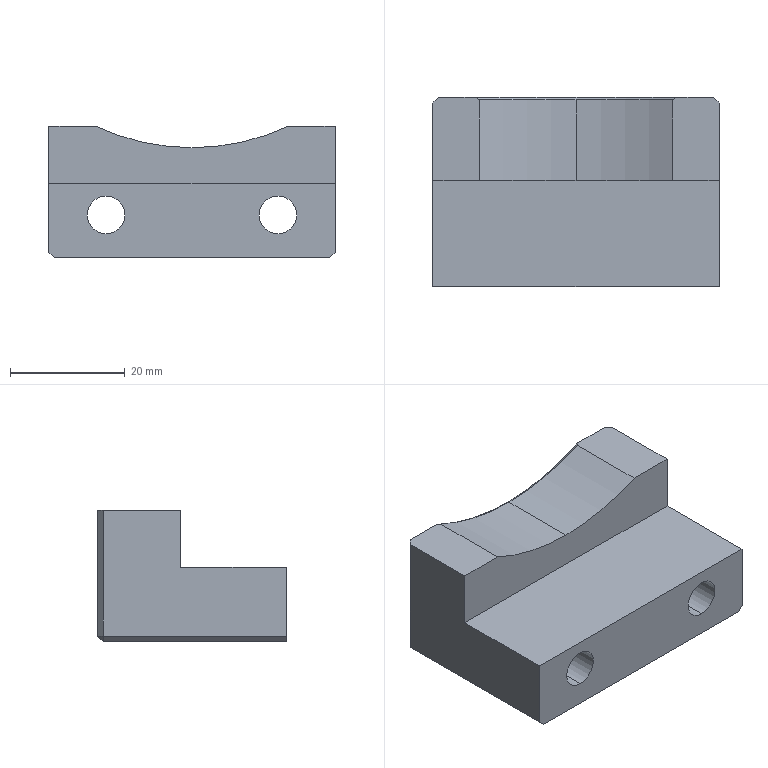Part | STEP file | PN_0004 Default | 1 solid | 29 faces | box 50 x 33 x 23 mm | volume 24275 mm3 | plane 18 | cylinder 10 | cone 1 | commonest cylinder face diameters 6.6 x4 11 x4 79.5 x2
STEP:
#1=CARTESIAN_POINT('',(16.854,32.57,3.));
#2=VERTEX_POINT('',#1);
#3=CARTESIAN_POINT('',(0.,32.57,-0.75));
#4=VERTEX_POINT('',#3);
#5=CARTESIAN_POINT('',(0.,32.57,39.));
#6=DIRECTION('',(0.,1.,0.));
#7=DIRECTION('',(0.,0.,-1.));
#8=AXIS2_PLACEMENT_3D('',#5,#6,#7);
#9=CIRCLE('',#8,39.75);
#10=EDGE_CURVE('',#2,#4,#9,.T.);
#11=ORIENTED_EDGE('',*,*,#10,.T.);
#12=CARTESIAN_POINT('',(0.,18.5,-0.75));
#13=VERTEX_POINT('',#12);
#14=CARTESIAN_POINT('',(0.,77.5,-0.75));
#15=DIRECTION('',(0.,-1.,0.));
#16=VECTOR('',#15,1000.);
#17=LINE('',#14,#16);
#18=EDGE_CURVE('',#4,#13,#17,.T.);
#19=ORIENTED_EDGE('',*,*,#18,.T.);
#20=CARTESIAN_POINT('',(16.854,18.5,3.));
#21=VERTEX_POINT('',#20);
#22=CARTESIAN_POINT('',(0.,18.5,39.));
#23=DIRECTION('',(0.,-1.,0.));
#24=DIRECTION('',(0.,0.,-1.));
#25=AXIS2_PLACEMENT_3D('',#22,#23,#24);
#26=CIRCLE('',#25,39.75);
#27=EDGE_CURVE('',#13,#21,#26,.T.);
#28=ORIENTED_EDGE('',*,*,#27,.T.);
#29=CARTESIAN_POINT('',(16.854,77.5,3.));
#30=DIRECTION('',(0.,-1.,0.));
#31=VECTOR('',#30,1000.);
#32=LINE('',#29,#31);
#33=EDGE_CURVE('',#2,#21,#32,.T.);
#34=ORIENTED_EDGE('',*,*,#33,.F.);
#35=EDGE_LOOP('',(#11,#19,#28,#34));
#36=FACE_OUTER_BOUND('',#35,.T.);
#37=CARTESIAN_POINT('',(0.,77.5,39.));
#38=DIRECTION('',(0.,-1.,0.));
#39=DIRECTION('',(0.,0.,-1.));
#40=AXIS2_PLACEMENT_3D('',#37,#38,#39);
#41=CYLINDRICAL_SURFACE('',#40,39.75);
#42=ADVANCED_FACE('',(#36),#41,.F.);
#43=CARTESIAN_POINT('',(-15.,26.,-18.));
#44=VERTEX_POINT('',#43);
#45=CARTESIAN_POINT('',(-15.,26.,-7.));
#46=VERTEX_POINT('',#45);
#47=CARTESIAN_POINT('',(-15.,26.,-12.5));
#48=DIRECTION('',(0.,1.,0.));
#49=DIRECTION('',(0.,0.,1.));
#50=AXIS2_PLACEMENT_3D('',#47,#48,#49);
#51=CIRCLE('',#50,5.5);
#52=EDGE_CURVE('',#44,#46,#51,.T.);
#53=ORIENTED_EDGE('',*,*,#52,.F.);
#54=CARTESIAN_POINT('',(-15.,33.,-18.));
#55=VERTEX_POINT('',#54);
#56=CARTESIAN_POINT('',(-15.,33.,-18.));
#57=DIRECTION('',(0.,1.,0.));
#58=VECTOR('',#57,1000.);
#59=LINE('',#56,#58);
#60=EDGE_CURVE('',#44,#55,#59,.T.);
#61=ORIENTED_EDGE('',*,*,#60,.T.);
#62=CARTESIAN_POINT('',(-15.,33.,-7.));
#63=VERTEX_POINT('',#62);
#64=CARTESIAN_POINT('',(-15.,33.,-12.5));
#65=DIRECTION('',(0.,1.,0.));
#66=DIRECTION('',(0.,0.,1.));
#67=AXIS2_PLACEMENT_3D('',#64,#65,#66);
#68=CIRCLE('',#67,5.5);
#69=EDGE_CURVE('',#55,#63,#68,.T.);
#70=ORIENTED_EDGE('',*,*,#69,.T.);
#71=CARTESIAN_POINT('',(-15.,33.,-7.));
#72=DIRECTION('',(0.,1.,0.));
#73=VECTOR('',#72,1000.);
#74=LINE('',#71,#73);
#75=EDGE_CURVE('',#46,#63,#74,.T.);
#76=ORIENTED_EDGE('',*,*,#75,.F.);
#77=EDGE_LOOP('',(#53,#61,#70,#76));
#78=FACE_OUTER_BOUND('',#77,.T.);
#79=CARTESIAN_POINT('',(-15.,33.,-12.5));
#80=DIRECTION('',(0.,1.,0.));
#81=DIRECTION('',(0.,0.,1.));
#82=AXIS2_PLACEMENT_3D('',#79,#80,#81);
#83=CYLINDRICAL_SURFACE('',#82,5.5);
#84=ADVANCED_FACE('',(#78),#83,.F.);
#85=CARTESIAN_POINT('',(-15.,0.,-15.8));
#86=VERTEX_POINT('',#85);
#87=CARTESIAN_POINT('',(-15.,0.,-9.2));
#88=VERTEX_POINT('',#87);
#89=CARTESIAN_POINT('',(-15.,0.,-12.5));
#90=DIRECTION('',(0.,1.,0.));
#91=DIRECTION('',(0.,0.,1.));
#92=AXIS2_PLACEMENT_3D('',#89,#90,#91);
#93=CIRCLE('',#92,3.3);
#94=EDGE_CURVE('',#86,#88,#93,.T.);
#95=ORIENTED_EDGE('',*,*,#94,.F.);
#96=CARTESIAN_POINT('',(-15.,26.,-15.8));
#97=VERTEX_POINT('',#96);
#98=CARTESIAN_POINT('',(-15.,33.,-15.8));
#99=DIRECTION('',(0.,1.,0.));
#100=VECTOR('',#99,1000.);
#101=LINE('',#98,#100);
#102=EDGE_CURVE('',#86,#97,#101,.T.);
#103=ORIENTED_EDGE('',*,*,#102,.T.);
#104=CARTESIAN_POINT('',(-15.,26.,-9.2));
#105=VERTEX_POINT('',#104);
#106=CARTESIAN_POINT('',(-15.,26.,-12.5));
#107=DIRECTION('',(0.,1.,0.));
#108=DIRECTION('',(0.,0.,1.));
#109=AXIS2_PLACEMENT_3D('',#106,#107,#108);
#110=CIRCLE('',#109,3.3);
#111=EDGE_CURVE('',#97,#105,#110,.T.);
#112=ORIENTED_EDGE('',*,*,#111,.T.);
#113=CARTESIAN_POINT('',(-15.,33.,-9.2));
#114=DIRECTION('',(0.,1.,0.));
#115=VECTOR('',#114,1000.);
#116=LINE('',#113,#115);
#117=EDGE_CURVE('',#88,#105,#116,.T.);
#118=ORIENTED_EDGE('',*,*,#117,.F.);
#119=EDGE_LOOP('',(#95,#103,#112,#118));
#120=FACE_OUTER_BOUND('',#119,.T.);
#121=CARTESIAN_POINT('',(-15.,33.,-12.5));
#122=DIRECTION('',(0.,1.,0.));
#123=DIRECTION('',(0.,0.,1.));
#124=AXIS2_PLACEMENT_3D('',#121,#122,#123);
#125=CYLINDRICAL_SURFACE('',#124,3.3);
#126=ADVANCED_FACE('',(#120),#125,.F.);
#127=CARTESIAN_POINT('',(15.,26.,-18.));
#128=VERTEX_POINT('',#127);
#129=CARTESIAN_POINT('',(15.,26.,-7.));
#130=VERTEX_POINT('',#129);
#131=CARTESIAN_POINT('',(15.,26.,-12.5));
#132=DIRECTION('',(0.,1.,0.));
#133=DIRECTION('',(0.,0.,1.));
#134=AXIS2_PLACEMENT_3D('',#131,#132,#133);
#135=CIRCLE('',#134,5.5);
#136=EDGE_CURVE('',#128,#130,#135,.T.);
#137=ORIENTED_EDGE('',*,*,#136,.F.);
#138=CARTESIAN_POINT('',(15.,33.,-18.));
#139=VERTEX_POINT('',#138);
#140=CARTESIAN_POINT('',(15.,33.,-18.));
#141=DIRECTION('',(0.,1.,0.));
#142=VECTOR('',#141,1000.);
#143=LINE('',#140,#142);
#144=EDGE_CURVE('',#128,#139,#143,.T.);
#145=ORIENTED_EDGE('',*,*,#144,.T.);
#146=CARTESIAN_POINT('',(15.,33.,-7.));
#147=VERTEX_POINT('',#146);
#148=CARTESIAN_POINT('',(15.,33.,-12.5));
#149=DIRECTION('',(0.,1.,0.));
#150=DIRECTION('',(0.,0.,1.));
#151=AXIS2_PLACEMENT_3D('',#148,#149,#150);
#152=CIRCLE('',#151,5.5);
#153=EDGE_CURVE('',#139,#147,#152,.T.);
#154=ORIENTED_EDGE('',*,*,#153,.T.);
#155=CARTESIAN_POINT('',(15.,33.,-7.));
#156=DIRECTION('',(0.,1.,0.));
#157=VECTOR('',#156,1000.);
#158=LINE('',#155,#157);
#159=EDGE_CURVE('',#130,#147,#158,.T.);
#160=ORIENTED_EDGE('',*,*,#159,.F.);
#161=EDGE_LOOP('',(#137,#145,#154,#160));
#162=FACE_OUTER_BOUND('',#161,.T.);
#163=CARTESIAN_POINT('',(15.,33.,-12.5));
#164=DIRECTION('',(0.,1.,0.));
#165=DIRECTION('',(0.,0.,1.));
#166=AXIS2_PLACEMENT_3D('',#163,#164,#165);
#167=CYLINDRICAL_SURFACE('',#166,5.5);
#168=ADVANCED_FACE('',(#162),#167,.F.);
#169=CARTESIAN_POINT('',(15.,0.,-15.8));
#170=VERTEX_POINT('',#169);
#171=CARTESIAN_POINT('',(15.,0.,-9.2));
#172=VERTEX_POINT('',#171);
#173=CARTESIAN_POINT('',(15.,0.,-12.5));
#174=DIRECTION('',(0.,1.,0.));
#175=DIRECTION('',(0.,0.,1.));
#176=AXIS2_PLACEMENT_3D('',#173,#174,#175);
#177=CIRCLE('',#176,3.3);
#178=EDGE_CURVE('',#170,#172,#177,.T.);
#179=ORIENTED_EDGE('',*,*,#178,.F.);
#180=CARTESIAN_POINT('',(15.,26.,-15.8));
#181=VERTEX_POINT('',#180);
#182=CARTESIAN_POINT('',(15.,33.,-15.8));
#183=DIRECTION('',(0.,1.,0.));
#184=VECTOR('',#183,1000.);
#185=LINE('',#182,#184);
#186=EDGE_CURVE('',#170,#181,#185,.T.);
#187=ORIENTED_EDGE('',*,*,#186,.T.);
#188=CARTESIAN_POINT('',(15.,26.,-9.2));
#189=VERTEX_POINT('',#188);
#190=CARTESIAN_POINT('',(15.,26.,-12.5));
#191=DIRECTION('',(0.,1.,0.));
#192=DIRECTION('',(0.,0.,1.));
#193=AXIS2_PLACEMENT_3D('',#190,#191,#192);
#194=CIRCLE('',#193,3.3);
#195=EDGE_CURVE('',#181,#189,#194,.T.);
#196=ORIENTED_EDGE('',*,*,#195,.T.);
#197=CARTESIAN_POINT('',(15.,33.,-9.2));
#198=DIRECTION('',(0.,1.,0.));
#199=VECTOR('',#198,1000.);
#200=LINE('',#197,#199);
#201=EDGE_CURVE('',#172,#189,#200,.T.);
#202=ORIENTED_EDGE('',*,*,#201,.F.);
#203=EDGE_LOOP('',(#179,#187,#196,#202));
#204=FACE_OUTER_BOUND('',#203,.T.);
#205=CARTESIAN_POINT('',(15.,33.,-12.5));
#206=DIRECTION('',(0.,1.,0.));
#207=DIRECTION('',(0.,0.,1.));
#208=AXIS2_PLACEMENT_3D('',#205,#206,#207);
#209=CYLINDRICAL_SURFACE('',#208,3.3);
#210=ADVANCED_FACE('',(#204),#209,.F.);
#211=CARTESIAN_POINT('',(24.,33.,3.));
#212=VERTEX_POINT('',#211);
#213=CARTESIAN_POINT('',(17.432,33.,3.));
#214=VERTEX_POINT('',#213);
#215=CARTESIAN_POINT('',(-25.,33.,3.));
#216=DIRECTION('',(-1.,0.,0.));
#217=VECTOR('',#216,1000.);
#218=LINE('',#215,#217);
#219=EDGE_CURVE('',#212,#214,#218,.T.);
#220=ORIENTED_EDGE('',*,*,#219,.T.);
#221=CARTESIAN_POINT('',(17.432,33.,3.));
#222=CARTESIAN_POINT('',(17.24,32.855,3.));
#223=CARTESIAN_POINT('',(17.048,32.712,3.));
#224=CARTESIAN_POINT('',(16.854,32.57,3.));
#225=B_SPLINE_CURVE_WITH_KNOTS('',3,(#221,#222,#223,#224),.UNSPECIFIED.,.F.,.F.,(4,4),(0.,0.00072),.UNSPECIFIED.);
#226=EDGE_CURVE('',#214,#2,#225,.T.);
#227=ORIENTED_EDGE('',*,*,#226,.T.);
#228=ORIENTED_EDGE('',*,*,#33,.T.);
#229=CARTESIAN_POINT('',(25.,18.5,3.));
#230=VERTEX_POINT('',#229);
#231=CARTESIAN_POINT('',(-25.,18.5,3.));
#232=DIRECTION('',(1.,0.,0.));
#233=VECTOR('',#232,1000.);
#234=LINE('',#231,#233);
#235=EDGE_CURVE('',#21,#230,#234,.T.);
#236=ORIENTED_EDGE('',*,*,#235,.T.);
#237=CARTESIAN_POINT('',(25.,32.,3.));
#238=VERTEX_POINT('',#237);
#239=CARTESIAN_POINT('',(25.,18.5,3.));
#240=DIRECTION('',(0.,1.,0.));
#241=VECTOR('',#240,1000.);
#242=LINE('',#239,#241);
#243=EDGE_CURVE('',#230,#238,#242,.T.);
#244=ORIENTED_EDGE('',*,*,#243,.T.);
#245=CARTESIAN_POINT('',(24.,33.,3.));
#246=DIRECTION('',(-0.7071,0.7071,0.));
#247=VECTOR('',#246,1000.);
#248=LINE('',#245,#247);
#249=EDGE_CURVE('',#238,#212,#248,.T.);
#250=ORIENTED_EDGE('',*,*,#249,.T.);
#251=EDGE_LOOP('',(#220,#227,#228,#236,#244,#250));
#252=FACE_OUTER_BOUND('',#251,.T.);
#253=CARTESIAN_POINT('',(0.,0.,3.));
#254=DIRECTION('',(0.,0.,-1.));
#255=DIRECTION('',(-1.,0.,0.));
#256=AXIS2_PLACEMENT_3D('',#253,#254,#255);
#257=PLANE('',#256);
#258=ADVANCED_FACE('',(#252),#257,.F.);
#259=CARTESIAN_POINT('',(-25.,32.,3.));
#260=VERTEX_POINT('',#259);
#261=CARTESIAN_POINT('',(-25.,18.5,3.));
#262=VERTEX_POINT('',#261);
#263=CARTESIAN_POINT('',(-25.,18.5,3.));
#264=DIRECTION('',(0.,-1.,0.));
#265=VECTOR('',#264,1000.);
#266=LINE('',#263,#265);
#267=EDGE_CURVE('',#260,#262,#266,.T.);
#268=ORIENTED_EDGE('',*,*,#267,.F.);
#269=CARTESIAN_POINT('',(-25.,32.,-19.));
#270=VERTEX_POINT('',#269);
#271=CARTESIAN_POINT('',(-25.,32.,0.));
#272=DIRECTION('',(0.,0.,-1.));
#273=VECTOR('',#272,1000.);
#274=LINE('',#271,#273);
#275=EDGE_CURVE('',#260,#270,#274,.T.);
#276=ORIENTED_EDGE('',*,*,#275,.T.);
#277=CARTESIAN_POINT('',(-25.,0.,-19.));
#278=VERTEX_POINT('',#277);
#279=CARTESIAN_POINT('',(-25.,33.,-19.));
#280=DIRECTION('',(0.,-1.,0.));
#281=VECTOR('',#280,1000.);
#282=LINE('',#279,#281);
#283=EDGE_CURVE('',#270,#278,#282,.T.);
#284=ORIENTED_EDGE('',*,*,#283,.T.);
#285=CARTESIAN_POINT('',(-25.,0.,-7.));
#286=VERTEX_POINT('',#285);
#287=CARTESIAN_POINT('',(-25.,0.,0.));
#288=DIRECTION('',(0.,0.,1.));
#289=VECTOR('',#288,1000.);
#290=LINE('',#287,#289);
#291=EDGE_CURVE('',#278,#286,#290,.T.);
#292=ORIENTED_EDGE('',*,*,#291,.T.);
#293=CARTESIAN_POINT('',(-25.,18.5,-7.));
#294=VERTEX_POINT('',#293);
#295=CARTESIAN_POINT('',(-25.,33.,-7.));
#296=DIRECTION('',(0.,1.,0.));
#297=VECTOR('',#296,1000.);
#298=LINE('',#295,#297);
#299=EDGE_CURVE('',#286,#294,#298,.T.);
#300=ORIENTED_EDGE('',*,*,#299,.T.);
#301=CARTESIAN_POINT('',(-25.,18.5,3.));
#302=DIRECTION('',(0.,0.,-1.));
#303=VECTOR('',#302,1000.);
#304=LINE('',#301,#303);
#305=EDGE_CURVE('',#262,#294,#304,.T.);
#306=ORIENTED_EDGE('',*,*,#305,.F.);
#307=EDGE_LOOP('',(#268,#276,#284,#292,#300,#306));
#308=FACE_OUTER_BOUND('',#307,.T.);
#309=CARTESIAN_POINT('',(-25.,33.,0.));
#310=DIRECTION('',(1.,0.,0.));
#311=DIRECTION('',(0.,0.,-1.));
#312=AXIS2_PLACEMENT_3D('',#309,#310,#311);
#313=PLANE('',#312);
#314=ADVANCED_FACE('',(#308),#313,.F.);
#315=CARTESIAN_POINT('',(25.,0.,-19.));
#316=VERTEX_POINT('',#315);
#317=CARTESIAN_POINT('',(25.,32.,-19.));
#318=VERTEX_POINT('',#317);
#319=CARTESIAN_POINT('',(25.,33.,-19.));
#320=DIRECTION('',(0.,1.,0.));
#321=VECTOR('',#320,1000.);
#322=LINE('',#319,#321);
#323=EDGE_CURVE('',#316,#318,#322,.T.);
#324=ORIENTED_EDGE('',*,*,#323,.T.);
#325=CARTESIAN_POINT('',(25.,32.,0.));
#326=DIRECTION('',(0.,0.,1.));
#327=VECTOR('',#326,1000.);
#328=LINE('',#325,#327);
#329=EDGE_CURVE('',#318,#238,#328,.T.);
#330=ORIENTED_EDGE('',*,*,#329,.T.);
#331=ORIENTED_EDGE('',*,*,#243,.F.);
#332=CARTESIAN_POINT('',(25.,18.5,-7.));
#333=VERTEX_POINT('',#332);
#334=CARTESIAN_POINT('',(25.,18.5,3.));
#335=DIRECTION('',(0.,0.,-1.));
#336=VECTOR('',#335,1000.);
#337=LINE('',#334,#336);
#338=EDGE_CURVE('',#230,#333,#337,.T.);
#339=ORIENTED_EDGE('',*,*,#338,.T.);
#340=CARTESIAN_POINT('',(25.,0.,-7.));
#341=VERTEX_POINT('',#340);
#342=CARTESIAN_POINT('',(25.,33.,-7.));
#343=DIRECTION('',(0.,-1.,0.));
#344=VECTOR('',#343,1000.);
#345=LINE('',#342,#344);
#346=EDGE_CURVE('',#333,#341,#345,.T.);
#347=ORIENTED_EDGE('',*,*,#346,.T.);
#348=CARTESIAN_POINT('',(25.,0.,0.));
#349=DIRECTION('',(0.,0.,-1.));
#350=VECTOR('',#349,1000.);
#351=LINE('',#348,#350);
#352=EDGE_CURVE('',#341,#316,#351,.T.);
#353=ORIENTED_EDGE('',*,*,#352,.T.);
#354=EDGE_LOOP('',(#324,#330,#331,#339,#347,#353));
#355=FACE_OUTER_BOUND('',#354,.T.);
#356=CARTESIAN_POINT('',(25.,33.,0.));
#357=DIRECTION('',(-1.,0.,0.));
#358=DIRECTION('',(0.,0.,1.));
#359=AXIS2_PLACEMENT_3D('',#356,#357,#358);
#360=PLANE('',#359);
#361=ADVANCED_FACE('',(#355),#360,.F.);
#362=CARTESIAN_POINT('',(24.,0.,-20.));
#363=VERTEX_POINT('',#362);
#364=CARTESIAN_POINT('',(-24.,0.,-20.));
#365=VERTEX_POINT('',#364);
#366=CARTESIAN_POINT('',(-25.,0.,-20.));
#367=DIRECTION('',(-1.,0.,0.));
#368=VECTOR('',#367,1000.);
#369=LINE('',#366,#368);
#370=EDGE_CURVE('',#363,#365,#369,.T.);
#371=ORIENTED_EDGE('',*,*,#370,.T.);
#372=CARTESIAN_POINT('',(-24.,32.,-20.));
#373=VERTEX_POINT('',#372);
#374=CARTESIAN_POINT('',(-24.,33.,-20.));
#375=DIRECTION('',(0.,1.,0.));
#376=VECTOR('',#375,1000.);
#377=LINE('',#374,#376);
#378=EDGE_CURVE('',#365,#373,#377,.T.);
#379=ORIENTED_EDGE('',*,*,#378,.T.);
#380=CARTESIAN_POINT('',(24.,32.,-20.));
#381=VERTEX_POINT('',#380);
#382=CARTESIAN_POINT('',(-25.,32.,-20.));
#383=DIRECTION('',(1.,0.,0.));
#384=VECTOR('',#383,1000.);
#385=LINE('',#382,#384);
#386=EDGE_CURVE('',#373,#381,#385,.T.);
#387=ORIENTED_EDGE('',*,*,#386,.T.);
#388=CARTESIAN_POINT('',(24.,33.,-20.));
#389=DIRECTION('',(0.,-1.,0.));
#390=VECTOR('',#389,1000.);
#391=LINE('',#388,#390);
#392=EDGE_CURVE('',#381,#363,#391,.T.);
#393=ORIENTED_EDGE('',*,*,#392,.T.);
#394=EDGE_LOOP('',(#371,#379,#387,#393));
#395=FACE_OUTER_BOUND('',#394,.T.);
#396=CARTESIAN_POINT('',(-25.,33.,-20.));
#397=DIRECTION('',(0.,0.,1.));
#398=DIRECTION('',(1.,0.,0.));
#399=AXIS2_PLACEMENT_3D('',#396,#397,#398);
#400=PLANE('',#399);
#401=ADVANCED_FACE('',(#395),#400,.F.);
#402=CARTESIAN_POINT('',(-15.,33.,-12.5));
#403=DIRECTION('',(0.,1.,0.));
#404=DIRECTION('',(0.,0.,1.));
#405=AXIS2_PLACEMENT_3D('',#402,#403,#404);
#406=CIRCLE('',#405,5.5);
#407=EDGE_CURVE('',#63,#55,#406,.T.);
#408=ORIENTED_EDGE('',*,*,#407,.F.);
#409=ORIENTED_EDGE('',*,*,#69,.F.);
#410=EDGE_LOOP('',(#408,#409));
#411=FACE_BOUND('',#410,.T.);
#412=CARTESIAN_POINT('',(15.,33.,-12.5));
#413=DIRECTION('',(0.,1.,0.));
#414=DIRECTION('',(0.,0.,1.));
#415=AXIS2_PLACEMENT_3D('',#412,#413,#414);
#416=CIRCLE('',#415,5.5);
#417=EDGE_CURVE('',#147,#139,#416,.T.);
#418=ORIENTED_EDGE('',*,*,#417,.F.);
#419=ORIENTED_EDGE('',*,*,#153,.F.);
#420=EDGE_LOOP('',(#418,#419));
#421=FACE_BOUND('',#420,.T.);
#422=CARTESIAN_POINT('',(-17.432,33.,3.));
#423=VERTEX_POINT('',#422);
#424=CARTESIAN_POINT('',(-24.,33.,3.));
#425=VERTEX_POINT('',#424);
#426=CARTESIAN_POINT('',(-25.,33.,3.));
#427=DIRECTION('',(-1.,0.,0.));
#428=VECTOR('',#427,1000.);
#429=LINE('',#426,#428);
#430=EDGE_CURVE('',#423,#425,#429,.T.);
#431=ORIENTED_EDGE('',*,*,#430,.F.);
#432=CARTESIAN_POINT('',(0.,33.,39.));
#433=DIRECTION('',(0.,-1.,0.));
#434=DIRECTION('',(0.,0.,-1.));
#435=AXIS2_PLACEMENT_3D('',#432,#433,#434);
#436=CIRCLE('',#435,39.998);
#437=EDGE_CURVE('',#423,#214,#436,.T.);
#438=ORIENTED_EDGE('',*,*,#437,.T.);
#439=ORIENTED_EDGE('',*,*,#219,.F.);
#440=CARTESIAN_POINT('',(24.,33.,-19.));
#441=VERTEX_POINT('',#440);
#442=CARTESIAN_POINT('',(24.,33.,-20.));
#443=DIRECTION('',(0.,0.,-1.));
#444=VECTOR('',#443,1000.);
#445=LINE('',#442,#444);
#446=EDGE_CURVE('',#212,#441,#445,.T.);
#447=ORIENTED_EDGE('',*,*,#446,.T.);
#448=CARTESIAN_POINT('',(-24.,33.,-19.));
#449=VERTEX_POINT('',#448);
#450=CARTESIAN_POINT('',(-25.,33.,-19.));
#451=DIRECTION('',(-1.,0.,0.));
#452=VECTOR('',#451,1000.);
#453=LINE('',#450,#452);
#454=EDGE_CURVE('',#441,#449,#453,.T.);
#455=ORIENTED_EDGE('',*,*,#454,.T.);
#456=CARTESIAN_POINT('',(-24.,33.,-20.));
#457=DIRECTION('',(0.,0.,1.));
#458=VECTOR('',#457,1000.);
#459=LINE('',#456,#458);
#460=EDGE_CURVE('',#449,#425,#459,.T.);
#461=ORIENTED_EDGE('',*,*,#460,.T.);
#462=EDGE_LOOP('',(#431,#438,#439,#447,#455,#461));
#463=FACE_OUTER_BOUND('',#462,.T.);
#464=CARTESIAN_POINT('',(-25.,33.,-20.));
#465=DIRECTION('',(0.,-1.,0.));
#466=DIRECTION('',(0.,0.,-1.));
#467=AXIS2_PLACEMENT_3D('',#464,#465,#466);
#468=PLANE('',#467);
#469=ADVANCED_FACE('',(#411,#421,#463),#468,.F.);
#470=ORIENTED_EDGE('',*,*,#291,.F.);
#471=CARTESIAN_POINT('',(-24.5,0.,-19.5));
#472=DIRECTION('',(0.7071,0.,-0.7071));
#473=VECTOR('',#472,1000.);
#474=LINE('',#471,#473);
#475=EDGE_CURVE('',#278,#365,#474,.T.);
#476=ORIENTED_EDGE('',*,*,#475,.T.);
#477=ORIENTED_EDGE('',*,*,#370,.F.);
#478=CARTESIAN_POINT('',(-0.5,0.,-44.5));
#479=DIRECTION('',(0.7071,0.,0.7071));
#480=VECTOR('',#479,1000.);
#481=LINE('',#478,#480);
#482=EDGE_CURVE('',#363,#316,#481,.T.);
#483=ORIENTED_EDGE('',*,*,#482,.T.);
#484=ORIENTED_EDGE('',*,*,#352,.F.);
#485=CARTESIAN_POINT('',(-25.,0.,-7.));
#486=DIRECTION('',(1.,0.,0.));
#487=VECTOR('',#486,1000.);
#488=LINE('',#485,#487);
#489=EDGE_CURVE('',#286,#341,#488,.T.);
#490=ORIENTED_EDGE('',*,*,#489,.F.);
#491=EDGE_LOOP('',(#470,#476,#477,#483,#484,#490));
#492=FACE_OUTER_BOUND('',#491,.T.);
#493=CARTESIAN_POINT('',(-15.,0.,-12.5));
#494=DIRECTION('',(0.,1.,0.));
#495=DIRECTION('',(0.,0.,1.));
#496=AXIS2_PLACEMENT_3D('',#493,#494,#495);
#497=CIRCLE('',#496,3.3);
#498=EDGE_CURVE('',#88,#86,#497,.T.);
#499=ORIENTED_EDGE('',*,*,#498,.T.);
#500=ORIENTED_EDGE('',*,*,#94,.T.);
#501=EDGE_LOOP('',(#499,#500));
#502=FACE_BOUND('',#501,.T.);
#503=CARTESIAN_POINT('',(15.,0.,-12.5));
#504=DIRECTION('',(0.,1.,0.));
#505=DIRECTION('',(0.,0.,1.));
#506=AXIS2_PLACEMENT_3D('',#503,#504,#505);
#507=CIRCLE('',#506,3.3);
#508=EDGE_CURVE('',#172,#170,#507,.T.);
#509=ORIENTED_EDGE('',*,*,#508,.T.);
#510=ORIENTED_EDGE('',*,*,#178,.T.);
#511=EDGE_LOOP('',(#509,#510));
#512=FACE_BOUND('',#511,.T.);
#513=CARTESIAN_POINT('',(-25.,0.,-20.));
#514=DIRECTION('',(0.,-1.,0.));
#515=DIRECTION('',(0.,0.,-1.));
#516=AXIS2_PLACEMENT_3D('',#513,#514,#515);
#517=PLANE('',#516);
#518=ADVANCED_FACE('',(#492,#502,#512),#517,.T.);
#519=ORIENTED_EDGE('',*,*,#186,.F.);
#520=ORIENTED_EDGE('',*,*,#508,.F.);
#521=ORIENTED_EDGE('',*,*,#201,.T.);
#522=CARTESIAN_POINT('',(15.,26.,-12.5));
#523=DIRECTION('',(0.,1.,0.));
#524=DIRECTION('',(0.,0.,1.));
#525=AXIS2_PLACEMENT_3D('',#522,#523,#524);
#526=CIRCLE('',#525,3.3);
#527=EDGE_CURVE('',#189,#181,#526,.T.);
#528=ORIENTED_EDGE('',*,*,#527,.T.);
#529=EDGE_LOOP('',(#519,#520,#521,#528));
#530=FACE_OUTER_BOUND('',#529,.T.);
#531=CARTESIAN_POINT('',(15.,33.,-12.5));
#532=DIRECTION('',(0.,1.,0.));
#533=DIRECTION('',(0.,0.,1.));
#534=AXIS2_PLACEMENT_3D('',#531,#532,#533);
#535=CYLINDRICAL_SURFACE('',#534,3.3);
#536=ADVANCED_FACE('',(#530),#535,.F.);
#537=ORIENTED_EDGE('',*,*,#527,.F.);
#538=ORIENTED_EDGE('',*,*,#195,.F.);
#539=EDGE_LOOP('',(#537,#538));
#540=FACE_BOUND('',#539,.T.);
#541=CARTESIAN_POINT('',(15.,26.,-12.5));
#542=DIRECTION('',(0.,1.,0.));
#543=DIRECTION('',(0.,0.,1.));
#544=AXIS2_PLACEMENT_3D('',#541,#542,#543);
#545=CIRCLE('',#544,5.5);
#546=EDGE_CURVE('',#130,#128,#545,.T.);
#547=ORIENTED_EDGE('',*,*,#546,.T.);
#548=ORIENTED_EDGE('',*,*,#136,.T.);
#549=EDGE_LOOP('',(#547,#548));
#550=FACE_OUTER_BOUND('',#549,.T.);
#551=CARTESIAN_POINT('',(18.3,26.,-12.5));
#552=DIRECTION('',(0.,-1.,0.));
#553=DIRECTION('',(0.,0.,-1.));
#554=AXIS2_PLACEMENT_3D('',#551,#552,#553);
#555=PLANE('',#554);
#556=ADVANCED_FACE('',(#540,#550),#555,.F.);
#557=ORIENTED_EDGE('',*,*,#144,.F.);
#558=ORIENTED_EDGE('',*,*,#546,.F.);
#559=ORIENTED_EDGE('',*,*,#159,.T.);
#560=ORIENTED_EDGE('',*,*,#417,.T.);
#561=EDGE_LOOP('',(#557,#558,#559,#560));
#562=FACE_OUTER_BOUND('',#561,.T.);
#563=CARTESIAN_POINT('',(15.,33.,-12.5));
#564=DIRECTION('',(0.,1.,0.));
#565=DIRECTION('',(0.,0.,1.));
#566=AXIS2_PLACEMENT_3D('',#563,#564,#565);
#567=CYLINDRICAL_SURFACE('',#566,5.5);
#568=ADVANCED_FACE('',(#562),#567,.F.);
#569=ORIENTED_EDGE('',*,*,#102,.F.);
#570=ORIENTED_EDGE('',*,*,#498,.F.);
#571=ORIENTED_EDGE('',*,*,#117,.T.);
#572=CARTESIAN_POINT('',(-15.,26.,-12.5));
#573=DIRECTION('',(0.,1.,0.));
#574=DIRECTION('',(0.,0.,1.));
#575=AXIS2_PLACEMENT_3D('',#572,#573,#574);
#576=CIRCLE('',#575,3.3);
#577=EDGE_CURVE('',#105,#97,#576,.T.);
#578=ORIENTED_EDGE('',*,*,#577,.T.);
#579=EDGE_LOOP('',(#569,#570,#571,#578));
#580=FACE_OUTER_BOUND('',#579,.T.);
#581=CARTESIAN_POINT('',(-15.,33.,-12.5));
#582=DIRECTION('',(0.,1.,0.));
#583=DIRECTION('',(0.,0.,1.));
#584=AXIS2_PLACEMENT_3D('',#581,#582,#583);
#585=CYLINDRICAL_SURFACE('',#584,3.3);
#586=ADVANCED_FACE('',(#580),#585,.F.);
#587=ORIENTED_EDGE('',*,*,#577,.F.);
#588=ORIENTED_EDGE('',*,*,#111,.F.);
#589=EDGE_LOOP('',(#587,#588));
#590=FACE_BOUND('',#589,.T.);
#591=CARTESIAN_POINT('',(-15.,26.,-12.5));
#592=DIRECTION('',(0.,1.,0.));
#593=DIRECTION('',(0.,0.,1.));
#594=AXIS2_PLACEMENT_3D('',#591,#592,#593);
#595=CIRCLE('',#594,5.5);
#596=EDGE_CURVE('',#46,#44,#595,.T.);
#597=ORIENTED_EDGE('',*,*,#596,.T.);
#598=ORIENTED_EDGE('',*,*,#52,.T.);
#599=EDGE_LOOP('',(#597,#598));
#600=FACE_OUTER_BOUND('',#599,.T.);
#601=CARTESIAN_POINT('',(-11.7,26.,-12.5));
#602=DIRECTION('',(0.,-1.,0.));
#603=DIRECTION('',(0.,0.,-1.));
#604=AXIS2_PLACEMENT_3D('',#601,#602,#603);
#605=PLANE('',#604);
#606=ADVANCED_FACE('',(#590,#600),#605,.F.);
#607=ORIENTED_EDGE('',*,*,#60,.F.);
#608=ORIENTED_EDGE('',*,*,#596,.F.);
#609=ORIENTED_EDGE('',*,*,#75,.T.);
#610=ORIENTED_EDGE('',*,*,#407,.T.);
#611=EDGE_LOOP('',(#607,#608,#609,#610));
#612=FACE_OUTER_BOUND('',#611,.T.);
#613=CARTESIAN_POINT('',(-15.,33.,-12.5));
#614=DIRECTION('',(0.,1.,0.));
#615=DIRECTION('',(0.,0.,1.));
#616=AXIS2_PLACEMENT_3D('',#613,#614,#615);
#617=CYLINDRICAL_SURFACE('',#616,5.5);
#618=ADVANCED_FACE('',(#612),#617,.F.);
#619=ORIENTED_EDGE('',*,*,#235,.F.);
#620=ORIENTED_EDGE('',*,*,#27,.F.);
#621=CARTESIAN_POINT('',(-16.854,18.5,3.));
#622=VERTEX_POINT('',#621);
#623=CARTESIAN_POINT('',(0.,18.5,39.));
#624=DIRECTION('',(0.,-1.,0.));
#625=DIRECTION('',(0.,0.,-1.));
#626=AXIS2_PLACEMENT_3D('',#623,#624,#625);
#627=CIRCLE('',#626,39.75);
#628=EDGE_CURVE('',#622,#13,#627,.T.);
#629=ORIENTED_EDGE('',*,*,#628,.F.);
#630=CARTESIAN_POINT('',(-25.,18.5,3.));
#631=DIRECTION('',(1.,0.,0.));
#632=VECTOR('',#631,1000.);
#633=LINE('',#630,#632);
#634=EDGE_CURVE('',#262,#622,#633,.T.);
#635=ORIENTED_EDGE('',*,*,#634,.F.);
#636=ORIENTED_EDGE('',*,*,#305,.T.);
#637=CARTESIAN_POINT('',(32.081,18.5,-7.));
#638=DIRECTION('',(-1.,0.,0.));
#639=VECTOR('',#638,1000.);
#640=LINE('',#637,#639);
#641=EDGE_CURVE('',#333,#294,#640,.T.);
#642=ORIENTED_EDGE('',*,*,#641,.F.);
#643=ORIENTED_EDGE('',*,*,#338,.F.);
#644=EDGE_LOOP('',(#619,#620,#629,#635,#636,#642,#643));
#645=FACE_OUTER_BOUND('',#644,.T.);
#646=CARTESIAN_POINT('',(0.,18.5,39.));
#647=DIRECTION('',(0.,-1.,0.));
#648=DIRECTION('',(0.,0.,-1.));
#649=AXIS2_PLACEMENT_3D('',#646,#647,#648);
#650=PLANE('',#649);
#651=ADVANCED_FACE('',(#645),#650,.T.);
#652=CARTESIAN_POINT('',(-16.854,32.57,3.));
#653=VERTEX_POINT('',#652);
#654=CARTESIAN_POINT('',(-16.854,77.5,3.));
#655=DIRECTION('',(0.,1.,0.));
#656=VECTOR('',#655,1000.);
#657=LINE('',#654,#656);
#658=EDGE_CURVE('',#622,#653,#657,.T.);
#659=ORIENTED_EDGE('',*,*,#658,.T.);
#660=CARTESIAN_POINT('',(-16.854,32.57,3.));
#661=CARTESIAN_POINT('',(-17.048,32.712,3.));
#662=CARTESIAN_POINT('',(-17.24,32.855,3.));
#663=CARTESIAN_POINT('',(-17.432,33.,3.));
#664=B_SPLINE_CURVE_WITH_KNOTS('',3,(#660,#661,#662,#663),.UNSPECIFIED.,.F.,.F.,(4,4),(0.,0.00072),.UNSPECIFIED.);
#665=EDGE_CURVE('',#653,#423,#664,.T.);
#666=ORIENTED_EDGE('',*,*,#665,.T.);
#667=ORIENTED_EDGE('',*,*,#430,.T.);
#668=CARTESIAN_POINT('',(-24.,33.,3.));
#669=DIRECTION('',(-0.7071,-0.7071,0.));
#670=VECTOR('',#669,1000.);
#671=LINE('',#668,#670);
#672=EDGE_CURVE('',#425,#260,#671,.T.);
#673=ORIENTED_EDGE('',*,*,#672,.T.);
#674=ORIENTED_EDGE('',*,*,#267,.T.);
#675=ORIENTED_EDGE('',*,*,#634,.T.);
#676=EDGE_LOOP('',(#659,#666,#667,#673,#674,#675));
#677=FACE_OUTER_BOUND('',#676,.T.);
#678=CARTESIAN_POINT('',(0.,0.,3.));
#679=DIRECTION('',(0.,0.,-1.));
#680=DIRECTION('',(-1.,0.,0.));
#681=AXIS2_PLACEMENT_3D('',#678,#679,#680);
#682=PLANE('',#681);
#683=ADVANCED_FACE('',(#677),#682,.F.);
#684=ORIENTED_EDGE('',*,*,#18,.F.);
#685=CARTESIAN_POINT('',(0.,32.57,39.));
#686=DIRECTION('',(0.,1.,0.));
#687=DIRECTION('',(0.,0.,-1.));
#688=AXIS2_PLACEMENT_3D('',#685,#686,#687);
#689=CIRCLE('',#688,39.75);
#690=EDGE_CURVE('',#4,#653,#689,.T.);
#691=ORIENTED_EDGE('',*,*,#690,.T.);
#692=ORIENTED_EDGE('',*,*,#658,.F.);
#693=ORIENTED_EDGE('',*,*,#628,.T.);
#694=EDGE_LOOP('',(#684,#691,#692,#693));
#695=FACE_OUTER_BOUND('',#694,.T.);
#696=CARTESIAN_POINT('',(0.,77.5,39.));
#697=DIRECTION('',(0.,-1.,0.));
#698=DIRECTION('',(0.,0.,-1.));
#699=AXIS2_PLACEMENT_3D('',#696,#697,#698);
#700=CYLINDRICAL_SURFACE('',#699,39.75);
#701=ADVANCED_FACE('',(#695),#700,.F.);
#702=ORIENTED_EDGE('',*,*,#489,.T.);
#703=ORIENTED_EDGE('',*,*,#346,.F.);
#704=ORIENTED_EDGE('',*,*,#641,.T.);
#705=ORIENTED_EDGE('',*,*,#299,.F.);
#706=EDGE_LOOP('',(#702,#703,#704,#705));
#707=FACE_OUTER_BOUND('',#706,.T.);
#708=CARTESIAN_POINT('',(0.,0.,-7.));
#709=DIRECTION('',(0.,0.,-1.));
#710=DIRECTION('',(-1.,0.,0.));
#711=AXIS2_PLACEMENT_3D('',#708,#709,#710);
#712=PLANE('',#711);
#713=ADVANCED_FACE('',(#707),#712,.F.);
#714=ORIENTED_EDGE('',*,*,#482,.F.);
#715=ORIENTED_EDGE('',*,*,#392,.F.);
#716=CARTESIAN_POINT('',(24.5,32.,-19.5));
#717=DIRECTION('',(-0.7071,0.,-0.7071));
#718=VECTOR('',#717,1000.);
#719=LINE('',#716,#718);
#720=EDGE_CURVE('',#318,#381,#719,.T.);
#721=ORIENTED_EDGE('',*,*,#720,.F.);
#722=ORIENTED_EDGE('',*,*,#323,.F.);
#723=EDGE_LOOP('',(#714,#715,#721,#722));
#724=FACE_OUTER_BOUND('',#723,.T.);
#725=CARTESIAN_POINT('',(24.,33.,-20.));
#726=DIRECTION('',(-0.7071,0.,0.7071));
#727=DIRECTION('',(0.,-1.,0.));
#728=AXIS2_PLACEMENT_3D('',#725,#726,#727);
#729=PLANE('',#728);
#730=ADVANCED_FACE('',(#724),#729,.F.);
#731=ORIENTED_EDGE('',*,*,#249,.F.);
#732=ORIENTED_EDGE('',*,*,#329,.F.);
#733=CARTESIAN_POINT('',(24.,33.,-19.));
#734=DIRECTION('',(0.7071,-0.7071,0.));
#735=VECTOR('',#734,1000.);
#736=LINE('',#733,#735);
#737=EDGE_CURVE('',#441,#318,#736,.T.);
#738=ORIENTED_EDGE('',*,*,#737,.F.);
#739=ORIENTED_EDGE('',*,*,#446,.F.);
#740=EDGE_LOOP('',(#731,#732,#738,#739));
#741=FACE_OUTER_BOUND('',#740,.T.);
#742=CARTESIAN_POINT('',(24.,33.,-20.));
#743=DIRECTION('',(-0.7071,-0.7071,0.));
#744=DIRECTION('',(0.,0.,-1.));
#745=AXIS2_PLACEMENT_3D('',#742,#743,#744);
#746=PLANE('',#745);
#747=ADVANCED_FACE('',(#741),#746,.F.);
#748=ORIENTED_EDGE('',*,*,#737,.T.);
#749=ORIENTED_EDGE('',*,*,#720,.T.);
#750=CARTESIAN_POINT('',(24.,33.,-19.));
#751=DIRECTION('',(0.,-0.7071,-0.7071));
#752=VECTOR('',#751,1000.);
#753=LINE('',#750,#752);
#754=EDGE_CURVE('',#441,#381,#753,.T.);
#755=ORIENTED_EDGE('',*,*,#754,.F.);
#756=EDGE_LOOP('',(#748,#749,#755));
#757=FACE_OUTER_BOUND('',#756,.T.);
#758=CARTESIAN_POINT('',(24.,33.,-19.));
#759=DIRECTION('',(0.5774,0.5774,-0.5774));
#760=DIRECTION('',(-0.7071,0.7071,0.));
#761=AXIS2_PLACEMENT_3D('',#758,#759,#760);
#762=PLANE('',#761);
#763=ADVANCED_FACE('',(#757),#762,.T.);
#764=ORIENTED_EDGE('',*,*,#475,.F.);
#765=ORIENTED_EDGE('',*,*,#283,.F.);
#766=CARTESIAN_POINT('',(-25.,32.,-19.));
#767=DIRECTION('',(-0.7071,0.,0.7071));
#768=VECTOR('',#767,1000.);
#769=LINE('',#766,#768);
#770=EDGE_CURVE('',#373,#270,#769,.T.);
#771=ORIENTED_EDGE('',*,*,#770,.F.);
#772=ORIENTED_EDGE('',*,*,#378,.F.);
#773=EDGE_LOOP('',(#764,#765,#771,#772));
#774=FACE_OUTER_BOUND('',#773,.T.);
#775=CARTESIAN_POINT('',(-25.,33.,-19.));
#776=DIRECTION('',(0.7071,0.,0.7071));
#777=DIRECTION('',(0.,-1.,0.));
#778=AXIS2_PLACEMENT_3D('',#775,#776,#777);
#779=PLANE('',#778);
#780=ADVANCED_FACE('',(#774),#779,.F.);
#781=ORIENTED_EDGE('',*,*,#754,.T.);
#782=ORIENTED_EDGE('',*,*,#386,.F.);
#783=CARTESIAN_POINT('',(-24.,32.5,-19.5));
#784=DIRECTION('',(0.,-0.7071,-0.7071));
#785=VECTOR('',#784,1000.);
#786=LINE('',#783,#785);
#787=EDGE_CURVE('',#449,#373,#786,.T.);
#788=ORIENTED_EDGE('',*,*,#787,.F.);
#789=ORIENTED_EDGE('',*,*,#454,.F.);
#790=EDGE_LOOP('',(#781,#782,#788,#789));
#791=FACE_OUTER_BOUND('',#790,.T.);
#792=CARTESIAN_POINT('',(-25.,33.,-19.));
#793=DIRECTION('',(0.,-0.7071,0.7071));
#794=DIRECTION('',(-1.,0.,0.));
#795=AXIS2_PLACEMENT_3D('',#792,#793,#794);
#796=PLANE('',#795);
#797=ADVANCED_FACE('',(#791),#796,.F.);
#798=ORIENTED_EDGE('',*,*,#787,.T.);
#799=ORIENTED_EDGE('',*,*,#770,.T.);
#800=CARTESIAN_POINT('',(-25.,32.,-19.));
#801=DIRECTION('',(-0.7071,-0.7071,0.));
#802=VECTOR('',#801,1000.);
#803=LINE('',#800,#802);
#804=EDGE_CURVE('',#449,#270,#803,.T.);
#805=ORIENTED_EDGE('',*,*,#804,.F.);
#806=EDGE_LOOP('',(#798,#799,#805));
#807=FACE_OUTER_BOUND('',#806,.T.);
#808=CARTESIAN_POINT('',(-25.,32.,-19.));
#809=DIRECTION('',(-0.5774,0.5774,-0.5774));
#810=DIRECTION('',(-0.7071,-0.7071,0.));
#811=AXIS2_PLACEMENT_3D('',#808,#809,#810);
#812=PLANE('',#811);
#813=ADVANCED_FACE('',(#807),#812,.T.);
#814=ORIENTED_EDGE('',*,*,#804,.T.);
#815=ORIENTED_EDGE('',*,*,#275,.F.);
#816=ORIENTED_EDGE('',*,*,#672,.F.);
#817=ORIENTED_EDGE('',*,*,#460,.F.);
#818=EDGE_LOOP('',(#814,#815,#816,#817));
#819=FACE_OUTER_BOUND('',#818,.T.);
#820=CARTESIAN_POINT('',(-24.,33.,-20.));
#821=DIRECTION('',(0.7071,-0.7071,0.));
#822=DIRECTION('',(0.,0.,1.));
#823=AXIS2_PLACEMENT_3D('',#820,#821,#822);
#824=PLANE('',#823);
#825=ADVANCED_FACE('',(#819),#824,.F.);
#826=ORIENTED_EDGE('',*,*,#665,.F.);
#827=ORIENTED_EDGE('',*,*,#690,.F.);
#828=ORIENTED_EDGE('',*,*,#10,.F.);
#829=ORIENTED_EDGE('',*,*,#226,.F.);
#830=ORIENTED_EDGE('',*,*,#437,.F.);
#831=EDGE_LOOP('',(#826,#827,#828,#829,#830));
#832=FACE_OUTER_BOUND('',#831,.T.);
#833=CARTESIAN_POINT('',(0.,33.,39.));
#834=DIRECTION('',(0.,1.,0.));
#835=DIRECTION('',(0.,0.,1.));
#836=AXIS2_PLACEMENT_3D('',#833,#834,#835);
#837=CONICAL_SURFACE('',#836,39.998,0.5236);
#838=ADVANCED_FACE('',(#832),#837,.F.);
#839=CLOSED_SHELL('',(#42,#84,#126,#168,#210,#258,#314,#361,#401,#469,#518,#536,#556,#568,#586,#606,#618,#651,#683,#701,#713,#730,#747,#763,#780,#797,#813,#825,#838));
#840=MANIFOLD_SOLID_BREP('',#839);
#841=CARTESIAN_POINT('',(0.,0.,0.));
#842=DIRECTION('',(0.,0.,1.));
#843=DIRECTION('',(1.,0.,0.));
#844=AXIS2_PLACEMENT_3D('',#841,#842,#843);
#845=(LENGTH_UNIT()NAMED_UNIT(*)SI_UNIT(.MILLI.,.METRE.));
#846=UNCERTAINTY_MEASURE_WITH_UNIT(LENGTH_MEASURE(0.00001),#845,'','');
#847=(NAMED_UNIT(*)PLANE_ANGLE_UNIT()SI_UNIT($,.RADIAN.));
#848=(NAMED_UNIT(*)SI_UNIT($,.STERADIAN.)SOLID_ANGLE_UNIT());
#849=(GEOMETRIC_REPRESENTATION_CONTEXT(3)GLOBAL_UNCERTAINTY_ASSIGNED_CONTEXT((#846))GLOBAL_UNIT_ASSIGNED_CONTEXT((#845,#847,#848))REPRESENTATION_CONTEXT('',''));
#850=ADVANCED_BREP_SHAPE_REPRESENTATION('',(#840,#844),#849);